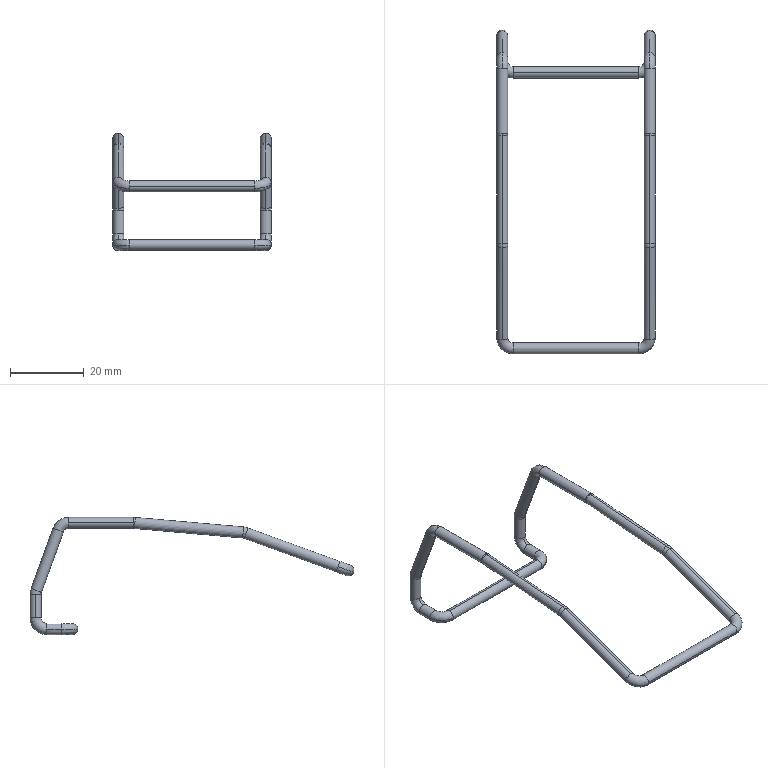Part | SolidWorks | features 3DProfileFeature 2, MirrorPattern 1, Sweep 1 | 1 solid | 56 faces | box 43 x 87.917 x 31.794 mm | volume 2200 mm3 | torus 28 | cylinder 28 | commonest cylinder face diameters 3 x28